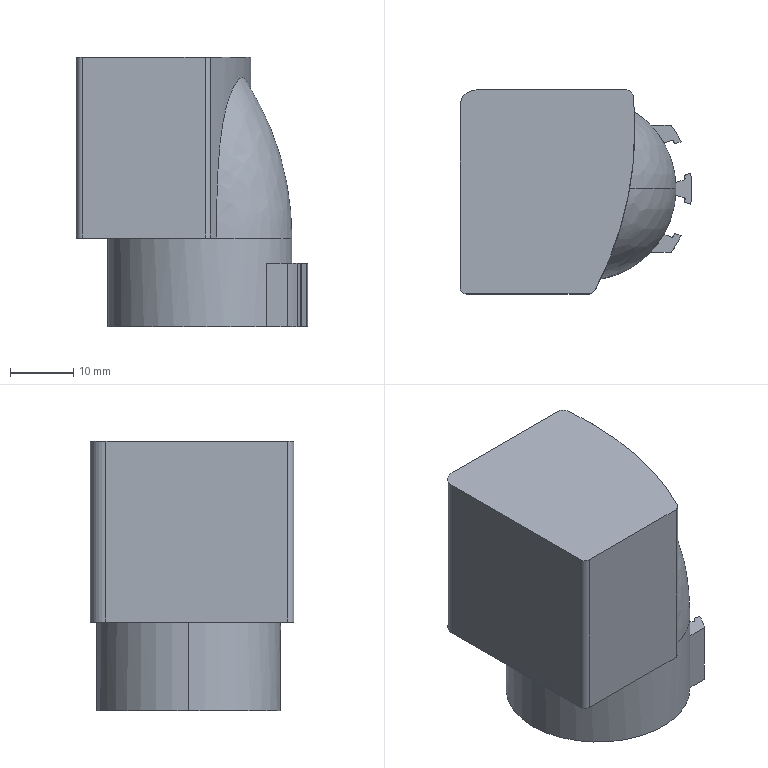Part | STEP file | P393261_cap_HMPL_16 | 1 solid | 60 faces | box 36.5 x 32.1 x 42.5 mm | volume 33239 mm3 | cylinder 34 | plane 22 | spline 2 | cone 2 | commonest cylinder face diameters 0.4 x10 0.8 x4 32 x4 34 x4 2 x3 12.8 x2